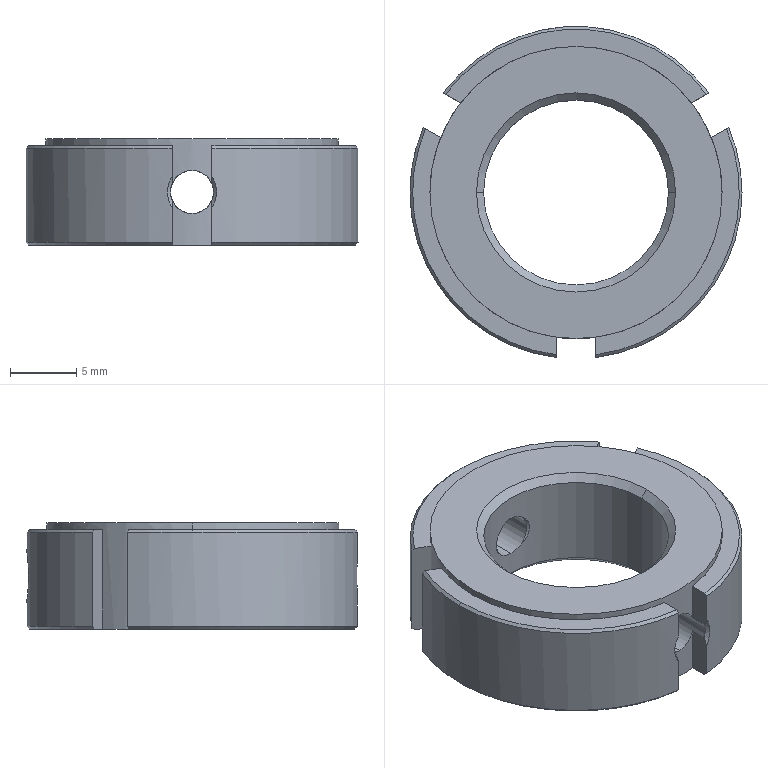Part | SolidWorks | features BaseBody 1 | 1 solid | 46 faces | box 25 x 24.91 x 8 mm | volume 2457 mm3 | cone 20 | cylinder 13 | plane 13 | commonest cylinder face diameters 3.242 x4 25 x4 22 x3 13.917 x2